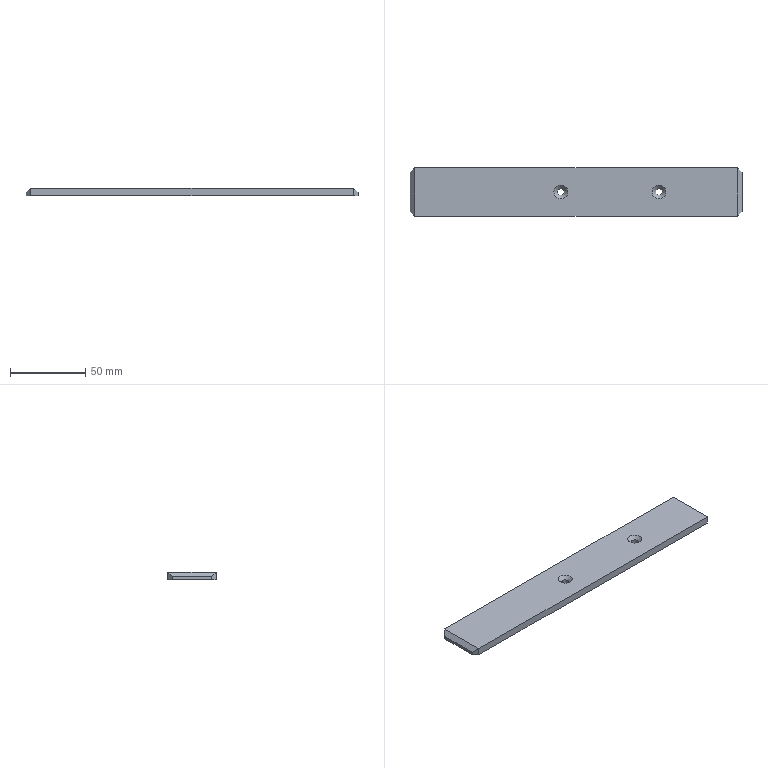Part | STEP file | Tube feed_id354_x_t | 1 solid | 16 faces | box 220 x 32 x 5 mm | volume 34590 mm3 | plane 12 | cone 2 | cylinder 2 | commonest cylinder face diameters 4.6 x2
STEP:
#1=CARTESIAN_POINT('',(0.,0.,0.));
#2=DIRECTION('',(0.,0.,1.));
#3=DIRECTION('',(1.,0.,0.));
#4=AXIS2_PLACEMENT_3D('',#1,#2,#3);
#5=CARTESIAN_POINT('',(203.,398.936,-4.));
#6=VERTEX_POINT('',#5);
#7=CARTESIAN_POINT('',(203.,424.936,-4.));
#8=VERTEX_POINT('',#7);
#9=CARTESIAN_POINT('',(203.,427.936,-4.));
#10=DIRECTION('',(0.,1.,0.));
#11=VECTOR('',#10,1.);
#12=LINE('',#9,#11);
#13=CARTESIAN_POINT('',(203.,427.936,-1.));
#14=DIRECTION('',(1.,0.,0.));
#15=DIRECTION('',(0.,0.,-1.));
#16=AXIS2_PLACEMENT_3D('',#13,#14,#15);
#17=PLANE('',#16);
#18=CARTESIAN_POINT('',(3.,0.));
#19=DIRECTION('',(0.,1.));
#20=VECTOR('',#19,1.);
#21=LINE('',#18,#20);
#22=(GEOMETRIC_REPRESENTATION_CONTEXT(2)PARAMETRIC_REPRESENTATION_CONTEXT()REPRESENTATION_CONTEXT('',''));
#23=DEFINITIONAL_REPRESENTATION('',(#21),#22);
#24=PCURVE('',#17,#23);
#25=CARTESIAN_POINT('',(206.,0.,-1.));
#26=DIRECTION('',(-0.7071,0.,0.7071));
#27=DIRECTION('',(0.,1.,0.));
#28=AXIS2_PLACEMENT_3D('',#25,#26,#27);
#29=PLANE('',#28);
#30=CARTESIAN_POINT('',(427.936,4.243));
#31=DIRECTION('',(1.,0.));
#32=VECTOR('',#31,1.);
#33=LINE('',#30,#32);
#34=(GEOMETRIC_REPRESENTATION_CONTEXT(2)PARAMETRIC_REPRESENTATION_CONTEXT()REPRESENTATION_CONTEXT('',''));
#35=DEFINITIONAL_REPRESENTATION('',(#33),#34);
#36=PCURVE('',#29,#35);
#37=SURFACE_CURVE('',#12,(#24,#36),.PCURVE_S1.);
#38=EDGE_CURVE('',#6,#8,#37,.T.);
#39=ORIENTED_EDGE('',*,*,#38,.T.);
#40=CARTESIAN_POINT('',(203.,424.936,-6.));
#41=VERTEX_POINT('',#40);
#42=CARTESIAN_POINT('',(203.,424.936,-1.));
#43=DIRECTION('',(0.,0.,-1.));
#44=VECTOR('',#43,1.);
#45=LINE('',#42,#44);
#46=CARTESIAN_POINT('',(0.,-3.));
#47=DIRECTION('',(1.,0.));
#48=VECTOR('',#47,1.);
#49=LINE('',#46,#48);
#50=(GEOMETRIC_REPRESENTATION_CONTEXT(2)PARAMETRIC_REPRESENTATION_CONTEXT()REPRESENTATION_CONTEXT('',''));
#51=DEFINITIONAL_REPRESENTATION('',(#49),#50);
#52=PCURVE('',#17,#51);
#53=CARTESIAN_POINT('',(203.,424.936,-1.));
#54=DIRECTION('',(0.7071,-0.7071,0.));
#55=DIRECTION('',(0.,0.,-1.));
#56=AXIS2_PLACEMENT_3D('',#53,#54,#55);
#57=PLANE('',#56);
#58=CARTESIAN_POINT('',(0.,0.));
#59=DIRECTION('',(1.,0.));
#60=VECTOR('',#59,1.);
#61=LINE('',#58,#60);
#62=(GEOMETRIC_REPRESENTATION_CONTEXT(2)PARAMETRIC_REPRESENTATION_CONTEXT()REPRESENTATION_CONTEXT('',''));
#63=DEFINITIONAL_REPRESENTATION('',(#61),#62);
#64=PCURVE('',#57,#63);
#65=SURFACE_CURVE('',#45,(#52,#64),.PCURVE_S1.);
#66=EDGE_CURVE('',#8,#41,#65,.T.);
#67=ORIENTED_EDGE('',*,*,#66,.T.);
#68=CARTESIAN_POINT('',(203.,398.936,-6.));
#69=VERTEX_POINT('',#68);
#70=CARTESIAN_POINT('',(203.,427.936,-6.));
#71=DIRECTION('',(0.,-1.,0.));
#72=VECTOR('',#71,1.);
#73=LINE('',#70,#72);
#74=CARTESIAN_POINT('',(5.,0.));
#75=DIRECTION('',(0.,-1.));
#76=VECTOR('',#75,1.);
#77=LINE('',#74,#76);
#78=(GEOMETRIC_REPRESENTATION_CONTEXT(2)PARAMETRIC_REPRESENTATION_CONTEXT()REPRESENTATION_CONTEXT('',''));
#79=DEFINITIONAL_REPRESENTATION('',(#77),#78);
#80=PCURVE('',#17,#79);
#81=CARTESIAN_POINT('',(0.,0.,-6.));
#82=DIRECTION('',(0.,0.,1.));
#83=DIRECTION('',(0.,-1.,0.));
#84=AXIS2_PLACEMENT_3D('',#81,#82,#83);
#85=PLANE('',#84);
#86=CARTESIAN_POINT('',(-427.936,203.));
#87=DIRECTION('',(1.,0.));
#88=VECTOR('',#87,1.);
#89=LINE('',#86,#88);
#90=(GEOMETRIC_REPRESENTATION_CONTEXT(2)PARAMETRIC_REPRESENTATION_CONTEXT()REPRESENTATION_CONTEXT('',''));
#91=DEFINITIONAL_REPRESENTATION('',(#89),#90);
#92=PCURVE('',#85,#91);
#93=SURFACE_CURVE('',#73,(#80,#92),.PCURVE_S1.);
#94=EDGE_CURVE('',#41,#69,#93,.T.);
#95=ORIENTED_EDGE('',*,*,#94,.T.);
#96=CARTESIAN_POINT('',(203.,398.936,-1.));
#97=DIRECTION('',(0.,0.,1.));
#98=VECTOR('',#97,1.);
#99=LINE('',#96,#98);
#100=CARTESIAN_POINT('',(0.,-29.));
#101=DIRECTION('',(-1.,0.));
#102=VECTOR('',#101,1.);
#103=LINE('',#100,#102);
#104=(GEOMETRIC_REPRESENTATION_CONTEXT(2)PARAMETRIC_REPRESENTATION_CONTEXT()REPRESENTATION_CONTEXT('',''));
#105=DEFINITIONAL_REPRESENTATION('',(#103),#104);
#106=PCURVE('',#17,#105);
#107=CARTESIAN_POINT('',(206.,395.936,-1.));
#108=DIRECTION('',(0.7071,0.7071,0.));
#109=DIRECTION('',(0.,0.,-1.));
#110=AXIS2_PLACEMENT_3D('',#107,#108,#109);
#111=PLANE('',#110);
#112=CARTESIAN_POINT('',(0.,4.243));
#113=DIRECTION('',(-1.,0.));
#114=VECTOR('',#113,1.);
#115=LINE('',#112,#114);
#116=(GEOMETRIC_REPRESENTATION_CONTEXT(2)PARAMETRIC_REPRESENTATION_CONTEXT()REPRESENTATION_CONTEXT('',''));
#117=DEFINITIONAL_REPRESENTATION('',(#115),#116);
#118=PCURVE('',#111,#117);
#119=SURFACE_CURVE('',#99,(#106,#118),.PCURVE_S1.);
#120=EDGE_CURVE('',#69,#6,#119,.T.);
#121=ORIENTED_EDGE('',*,*,#120,.T.);
#122=EDGE_LOOP('',(#39,#67,#95,#121));
#123=FACE_BOUND('',#122,.T.);
#124=ADVANCED_FACE('',(#123),#17,.F.);
#125=CARTESIAN_POINT('',(206.,395.936,-1.));
#126=VERTEX_POINT('',#125);
#127=CARTESIAN_POINT('',(420.,395.936,-1.));
#128=VERTEX_POINT('',#127);
#129=CARTESIAN_POINT('',(203.,395.936,-1.));
#130=DIRECTION('',(1.,0.,0.));
#131=VECTOR('',#130,1.);
#132=LINE('',#129,#131);
#133=CARTESIAN_POINT('',(203.,395.936,-1.));
#134=DIRECTION('',(0.,1.,0.));
#135=DIRECTION('',(0.,0.,1.));
#136=AXIS2_PLACEMENT_3D('',#133,#134,#135);
#137=PLANE('',#136);
#138=CARTESIAN_POINT('',(0.,0.));
#139=DIRECTION('',(0.,1.));
#140=VECTOR('',#139,1.);
#141=LINE('',#138,#140);
#142=(GEOMETRIC_REPRESENTATION_CONTEXT(2)PARAMETRIC_REPRESENTATION_CONTEXT()REPRESENTATION_CONTEXT('',''));
#143=DEFINITIONAL_REPRESENTATION('',(#141),#142);
#144=PCURVE('',#137,#143);
#145=CARTESIAN_POINT('',(0.,0.,-1.));
#146=DIRECTION('',(0.,0.,1.));
#147=DIRECTION('',(0.,-1.,0.));
#148=AXIS2_PLACEMENT_3D('',#145,#146,#147);
#149=PLANE('',#148);
#150=CARTESIAN_POINT('',(-395.936,203.));
#151=DIRECTION('',(0.,1.));
#152=VECTOR('',#151,1.);
#153=LINE('',#150,#152);
#154=(GEOMETRIC_REPRESENTATION_CONTEXT(2)PARAMETRIC_REPRESENTATION_CONTEXT()REPRESENTATION_CONTEXT('',''));
#155=DEFINITIONAL_REPRESENTATION('',(#153),#154);
#156=PCURVE('',#149,#155);
#157=SURFACE_CURVE('',#132,(#144,#156),.PCURVE_S1.);
#158=EDGE_CURVE('',#126,#128,#157,.T.);
#159=ORIENTED_EDGE('',*,*,#158,.F.);
#160=CARTESIAN_POINT('',(206.,395.936,-6.));
#161=VERTEX_POINT('',#160);
#162=CARTESIAN_POINT('',(206.,395.936,-1.));
#163=DIRECTION('',(0.,0.,-1.));
#164=VECTOR('',#163,1.);
#165=LINE('',#162,#164);
#166=CARTESIAN_POINT('',(0.,3.));
#167=DIRECTION('',(-1.,0.));
#168=VECTOR('',#167,1.);
#169=LINE('',#166,#168);
#170=(GEOMETRIC_REPRESENTATION_CONTEXT(2)PARAMETRIC_REPRESENTATION_CONTEXT()REPRESENTATION_CONTEXT('',''));
#171=DEFINITIONAL_REPRESENTATION('',(#169),#170);
#172=PCURVE('',#137,#171);
#173=CARTESIAN_POINT('',(0.,0.));
#174=DIRECTION('',(1.,0.));
#175=VECTOR('',#174,1.);
#176=LINE('',#173,#175);
#177=(GEOMETRIC_REPRESENTATION_CONTEXT(2)PARAMETRIC_REPRESENTATION_CONTEXT()REPRESENTATION_CONTEXT('',''));
#178=DEFINITIONAL_REPRESENTATION('',(#176),#177);
#179=PCURVE('',#111,#178);
#180=SURFACE_CURVE('',#165,(#172,#179),.PCURVE_S1.);
#181=EDGE_CURVE('',#126,#161,#180,.T.);
#182=ORIENTED_EDGE('',*,*,#181,.T.);
#183=CARTESIAN_POINT('',(420.,395.936,-6.));
#184=VERTEX_POINT('',#183);
#185=CARTESIAN_POINT('',(203.,395.936,-6.));
#186=DIRECTION('',(1.,0.,0.));
#187=VECTOR('',#186,1.);
#188=LINE('',#185,#187);
#189=CARTESIAN_POINT('',(-5.,0.));
#190=DIRECTION('',(0.,1.));
#191=VECTOR('',#190,1.);
#192=LINE('',#189,#191);
#193=(GEOMETRIC_REPRESENTATION_CONTEXT(2)PARAMETRIC_REPRESENTATION_CONTEXT()REPRESENTATION_CONTEXT('',''));
#194=DEFINITIONAL_REPRESENTATION('',(#192),#193);
#195=PCURVE('',#137,#194);
#196=CARTESIAN_POINT('',(-395.936,203.));
#197=DIRECTION('',(0.,1.));
#198=VECTOR('',#197,1.);
#199=LINE('',#196,#198);
#200=(GEOMETRIC_REPRESENTATION_CONTEXT(2)PARAMETRIC_REPRESENTATION_CONTEXT()REPRESENTATION_CONTEXT('',''));
#201=DEFINITIONAL_REPRESENTATION('',(#199),#200);
#202=PCURVE('',#85,#201);
#203=SURFACE_CURVE('',#188,(#195,#202),.PCURVE_S1.);
#204=EDGE_CURVE('',#161,#184,#203,.T.);
#205=ORIENTED_EDGE('',*,*,#204,.T.);
#206=CARTESIAN_POINT('',(420.,395.936,-1.));
#207=DIRECTION('',(0.,0.,1.));
#208=VECTOR('',#207,1.);
#209=LINE('',#206,#208);
#210=CARTESIAN_POINT('',(0.,217.));
#211=DIRECTION('',(1.,0.));
#212=VECTOR('',#211,1.);
#213=LINE('',#210,#212);
#214=(GEOMETRIC_REPRESENTATION_CONTEXT(2)PARAMETRIC_REPRESENTATION_CONTEXT()REPRESENTATION_CONTEXT('',''));
#215=DEFINITIONAL_REPRESENTATION('',(#213),#214);
#216=PCURVE('',#137,#215);
#217=CARTESIAN_POINT('',(423.,398.936,-1.));
#218=DIRECTION('',(-0.7071,0.7071,0.));
#219=DIRECTION('',(0.,0.,-1.));
#220=AXIS2_PLACEMENT_3D('',#217,#218,#219);
#221=PLANE('',#220);
#222=CARTESIAN_POINT('',(0.,4.243));
#223=DIRECTION('',(-1.,0.));
#224=VECTOR('',#223,1.);
#225=LINE('',#222,#224);
#226=(GEOMETRIC_REPRESENTATION_CONTEXT(2)PARAMETRIC_REPRESENTATION_CONTEXT()REPRESENTATION_CONTEXT('',''));
#227=DEFINITIONAL_REPRESENTATION('',(#225),#226);
#228=PCURVE('',#221,#227);
#229=SURFACE_CURVE('',#209,(#216,#228),.PCURVE_S1.);
#230=EDGE_CURVE('',#184,#128,#229,.T.);
#231=ORIENTED_EDGE('',*,*,#230,.T.);
#232=EDGE_LOOP('',(#159,#182,#205,#231));
#233=FACE_BOUND('',#232,.T.);
#234=ADVANCED_FACE('',(#233),#137,.F.);
#235=CARTESIAN_POINT('',(423.,398.936,-6.));
#236=VERTEX_POINT('',#235);
#237=CARTESIAN_POINT('',(423.,424.936,-6.));
#238=VERTEX_POINT('',#237);
#239=CARTESIAN_POINT('',(423.,395.936,-6.));
#240=DIRECTION('',(0.,1.,0.));
#241=VECTOR('',#240,1.);
#242=LINE('',#239,#241);
#243=CARTESIAN_POINT('',(423.,395.936,-1.));
#244=DIRECTION('',(-1.,0.,0.));
#245=DIRECTION('',(0.,0.,1.));
#246=AXIS2_PLACEMENT_3D('',#243,#244,#245);
#247=PLANE('',#246);
#248=CARTESIAN_POINT('',(-5.,0.));
#249=DIRECTION('',(0.,1.));
#250=VECTOR('',#249,1.);
#251=LINE('',#248,#250);
#252=(GEOMETRIC_REPRESENTATION_CONTEXT(2)PARAMETRIC_REPRESENTATION_CONTEXT()REPRESENTATION_CONTEXT('',''));
#253=DEFINITIONAL_REPRESENTATION('',(#251),#252);
#254=PCURVE('',#247,#253);
#255=CARTESIAN_POINT('',(-395.936,423.));
#256=DIRECTION('',(-1.,0.));
#257=VECTOR('',#256,1.);
#258=LINE('',#255,#257);
#259=(GEOMETRIC_REPRESENTATION_CONTEXT(2)PARAMETRIC_REPRESENTATION_CONTEXT()REPRESENTATION_CONTEXT('',''));
#260=DEFINITIONAL_REPRESENTATION('',(#258),#259);
#261=PCURVE('',#85,#260);
#262=SURFACE_CURVE('',#242,(#254,#261),.PCURVE_S1.);
#263=EDGE_CURVE('',#236,#238,#262,.T.);
#264=ORIENTED_EDGE('',*,*,#263,.T.);
#265=CARTESIAN_POINT('',(423.,424.936,-4.));
#266=VERTEX_POINT('',#265);
#267=CARTESIAN_POINT('',(423.,424.936,-1.));
#268=DIRECTION('',(0.,0.,1.));
#269=VECTOR('',#268,1.);
#270=LINE('',#267,#269);
#271=CARTESIAN_POINT('',(0.,29.));
#272=DIRECTION('',(1.,0.));
#273=VECTOR('',#272,1.);
#274=LINE('',#271,#273);
#275=(GEOMETRIC_REPRESENTATION_CONTEXT(2)PARAMETRIC_REPRESENTATION_CONTEXT()REPRESENTATION_CONTEXT('',''));
#276=DEFINITIONAL_REPRESENTATION('',(#274),#275);
#277=PCURVE('',#247,#276);
#278=CARTESIAN_POINT('',(420.,427.936,-1.));
#279=DIRECTION('',(-0.7071,-0.7071,0.));
#280=DIRECTION('',(0.,0.,-1.));
#281=AXIS2_PLACEMENT_3D('',#278,#279,#280);
#282=PLANE('',#281);
#283=CARTESIAN_POINT('',(0.,4.243));
#284=DIRECTION('',(-1.,0.));
#285=VECTOR('',#284,1.);
#286=LINE('',#283,#285);
#287=(GEOMETRIC_REPRESENTATION_CONTEXT(2)PARAMETRIC_REPRESENTATION_CONTEXT()REPRESENTATION_CONTEXT('',''));
#288=DEFINITIONAL_REPRESENTATION('',(#286),#287);
#289=PCURVE('',#282,#288);
#290=SURFACE_CURVE('',#270,(#277,#289),.PCURVE_S1.);
#291=EDGE_CURVE('',#238,#266,#290,.T.);
#292=ORIENTED_EDGE('',*,*,#291,.T.);
#293=CARTESIAN_POINT('',(423.,398.936,-4.));
#294=VERTEX_POINT('',#293);
#295=CARTESIAN_POINT('',(423.,395.936,-4.));
#296=DIRECTION('',(0.,-1.,0.));
#297=VECTOR('',#296,1.);
#298=LINE('',#295,#297);
#299=CARTESIAN_POINT('',(-3.,0.));
#300=DIRECTION('',(0.,-1.));
#301=VECTOR('',#300,1.);
#302=LINE('',#299,#301);
#303=(GEOMETRIC_REPRESENTATION_CONTEXT(2)PARAMETRIC_REPRESENTATION_CONTEXT()REPRESENTATION_CONTEXT('',''));
#304=DEFINITIONAL_REPRESENTATION('',(#302),#303);
#305=PCURVE('',#247,#304);
#306=CARTESIAN_POINT('',(420.,0.,-1.));
#307=DIRECTION('',(0.7071,0.,0.7071));
#308=DIRECTION('',(0.,-1.,0.));
#309=AXIS2_PLACEMENT_3D('',#306,#307,#308);
#310=PLANE('',#309);
#311=CARTESIAN_POINT('',(-395.936,4.243));
#312=DIRECTION('',(1.,0.));
#313=VECTOR('',#312,1.);
#314=LINE('',#311,#313);
#315=(GEOMETRIC_REPRESENTATION_CONTEXT(2)PARAMETRIC_REPRESENTATION_CONTEXT()REPRESENTATION_CONTEXT('',''));
#316=DEFINITIONAL_REPRESENTATION('',(#314),#315);
#317=PCURVE('',#310,#316);
#318=SURFACE_CURVE('',#298,(#305,#317),.PCURVE_S1.);
#319=EDGE_CURVE('',#266,#294,#318,.T.);
#320=ORIENTED_EDGE('',*,*,#319,.T.);
#321=CARTESIAN_POINT('',(423.,398.936,-1.));
#322=DIRECTION('',(0.,0.,-1.));
#323=VECTOR('',#322,1.);
#324=LINE('',#321,#323);
#325=CARTESIAN_POINT('',(0.,3.));
#326=DIRECTION('',(-1.,0.));
#327=VECTOR('',#326,1.);
#328=LINE('',#325,#327);
#329=(GEOMETRIC_REPRESENTATION_CONTEXT(2)PARAMETRIC_REPRESENTATION_CONTEXT()REPRESENTATION_CONTEXT('',''));
#330=DEFINITIONAL_REPRESENTATION('',(#328),#329);
#331=PCURVE('',#247,#330);
#332=CARTESIAN_POINT('',(0.,0.));
#333=DIRECTION('',(1.,0.));
#334=VECTOR('',#333,1.);
#335=LINE('',#332,#334);
#336=(GEOMETRIC_REPRESENTATION_CONTEXT(2)PARAMETRIC_REPRESENTATION_CONTEXT()REPRESENTATION_CONTEXT('',''));
#337=DEFINITIONAL_REPRESENTATION('',(#335),#336);
#338=PCURVE('',#221,#337);
#339=SURFACE_CURVE('',#324,(#331,#338),.PCURVE_S1.);
#340=EDGE_CURVE('',#294,#236,#339,.T.);
#341=ORIENTED_EDGE('',*,*,#340,.T.);
#342=EDGE_LOOP('',(#264,#292,#320,#341));
#343=FACE_BOUND('',#342,.T.);
#344=ADVANCED_FACE('',(#343),#247,.F.);
#345=CARTESIAN_POINT('',(420.,427.936,-6.));
#346=VERTEX_POINT('',#345);
#347=CARTESIAN_POINT('',(206.,427.936,-6.));
#348=VERTEX_POINT('',#347);
#349=CARTESIAN_POINT('',(423.,427.936,-6.));
#350=DIRECTION('',(-1.,0.,0.));
#351=VECTOR('',#350,1.);
#352=LINE('',#349,#351);
#353=CARTESIAN_POINT('',(423.,427.936,-1.));
#354=DIRECTION('',(0.,-1.,0.));
#355=DIRECTION('',(0.,0.,-1.));
#356=AXIS2_PLACEMENT_3D('',#353,#354,#355);
#357=PLANE('',#356);
#358=CARTESIAN_POINT('',(5.,0.));
#359=DIRECTION('',(0.,-1.));
#360=VECTOR('',#359,1.);
#361=LINE('',#358,#360);
#362=(GEOMETRIC_REPRESENTATION_CONTEXT(2)PARAMETRIC_REPRESENTATION_CONTEXT()REPRESENTATION_CONTEXT('',''));
#363=DEFINITIONAL_REPRESENTATION('',(#361),#362);
#364=PCURVE('',#357,#363);
#365=CARTESIAN_POINT('',(-427.936,423.));
#366=DIRECTION('',(0.,-1.));
#367=VECTOR('',#366,1.);
#368=LINE('',#365,#367);
#369=(GEOMETRIC_REPRESENTATION_CONTEXT(2)PARAMETRIC_REPRESENTATION_CONTEXT()REPRESENTATION_CONTEXT('',''));
#370=DEFINITIONAL_REPRESENTATION('',(#368),#369);
#371=PCURVE('',#85,#370);
#372=SURFACE_CURVE('',#352,(#364,#371),.PCURVE_S1.);
#373=EDGE_CURVE('',#346,#348,#372,.T.);
#374=ORIENTED_EDGE('',*,*,#373,.T.);
#375=CARTESIAN_POINT('',(206.,427.936,-1.));
#376=VERTEX_POINT('',#375);
#377=CARTESIAN_POINT('',(206.,427.936,-1.));
#378=DIRECTION('',(0.,0.,1.));
#379=VECTOR('',#378,1.);
#380=LINE('',#377,#379);
#381=CARTESIAN_POINT('',(0.,-217.));
#382=DIRECTION('',(-1.,0.));
#383=VECTOR('',#382,1.);
#384=LINE('',#381,#383);
#385=(GEOMETRIC_REPRESENTATION_CONTEXT(2)PARAMETRIC_REPRESENTATION_CONTEXT()REPRESENTATION_CONTEXT('',''));
#386=DEFINITIONAL_REPRESENTATION('',(#384),#385);
#387=PCURVE('',#357,#386);
#388=CARTESIAN_POINT('',(0.,4.243));
#389=DIRECTION('',(-1.,0.));
#390=VECTOR('',#389,1.);
#391=LINE('',#388,#390);
#392=(GEOMETRIC_REPRESENTATION_CONTEXT(2)PARAMETRIC_REPRESENTATION_CONTEXT()REPRESENTATION_CONTEXT('',''));
#393=DEFINITIONAL_REPRESENTATION('',(#391),#392);
#394=PCURVE('',#57,#393);
#395=SURFACE_CURVE('',#380,(#387,#394),.PCURVE_S1.);
#396=EDGE_CURVE('',#348,#376,#395,.T.);
#397=ORIENTED_EDGE('',*,*,#396,.T.);
#398=CARTESIAN_POINT('',(420.,427.936,-1.));
#399=VERTEX_POINT('',#398);
#400=CARTESIAN_POINT('',(423.,427.936,-1.));
#401=DIRECTION('',(-1.,0.,0.));
#402=VECTOR('',#401,1.);
#403=LINE('',#400,#402);
#404=CARTESIAN_POINT('',(0.,0.));
#405=DIRECTION('',(0.,-1.));
#406=VECTOR('',#405,1.);
#407=LINE('',#404,#406);
#408=(GEOMETRIC_REPRESENTATION_CONTEXT(2)PARAMETRIC_REPRESENTATION_CONTEXT()REPRESENTATION_CONTEXT('',''));
#409=DEFINITIONAL_REPRESENTATION('',(#407),#408);
#410=PCURVE('',#357,#409);
#411=CARTESIAN_POINT('',(-427.936,423.));
#412=DIRECTION('',(0.,-1.));
#413=VECTOR('',#412,1.);
#414=LINE('',#411,#413);
#415=(GEOMETRIC_REPRESENTATION_CONTEXT(2)PARAMETRIC_REPRESENTATION_CONTEXT()REPRESENTATION_CONTEXT('',''));
#416=DEFINITIONAL_REPRESENTATION('',(#414),#415);
#417=PCURVE('',#149,#416);
#418=SURFACE_CURVE('',#403,(#410,#417),.PCURVE_S1.);
#419=EDGE_CURVE('',#399,#376,#418,.T.);
#420=ORIENTED_EDGE('',*,*,#419,.F.);
#421=CARTESIAN_POINT('',(420.,427.936,-1.));
#422=DIRECTION('',(0.,0.,-1.));
#423=VECTOR('',#422,1.);
#424=LINE('',#421,#423);
#425=CARTESIAN_POINT('',(0.,-3.));
#426=DIRECTION('',(1.,0.));
#427=VECTOR('',#426,1.);
#428=LINE('',#425,#427);
#429=(GEOMETRIC_REPRESENTATION_CONTEXT(2)PARAMETRIC_REPRESENTATION_CONTEXT()REPRESENTATION_CONTEXT('',''));
#430=DEFINITIONAL_REPRESENTATION('',(#428),#429);
#431=PCURVE('',#357,#430);
#432=CARTESIAN_POINT('',(0.,0.));
#433=DIRECTION('',(1.,0.));
#434=VECTOR('',#433,1.);
#435=LINE('',#432,#434);
#436=(GEOMETRIC_REPRESENTATION_CONTEXT(2)PARAMETRIC_REPRESENTATION_CONTEXT()REPRESENTATION_CONTEXT('',''));
#437=DEFINITIONAL_REPRESENTATION('',(#435),#436);
#438=PCURVE('',#282,#437);
#439=SURFACE_CURVE('',#424,(#431,#438),.PCURVE_S1.);
#440=EDGE_CURVE('',#399,#346,#439,.T.);
#441=ORIENTED_EDGE('',*,*,#440,.T.);
#442=EDGE_LOOP('',(#374,#397,#420,#441));
#443=FACE_BOUND('',#442,.T.);
#444=ADVANCED_FACE('',(#443),#357,.F.);
#445=CARTESIAN_POINT('',(363.4,411.936,-1.));
#446=VERTEX_POINT('',#445);
#447=CARTESIAN_POINT('',(368.,411.936,-1.));
#448=DIRECTION('',(0.,0.,-1.));
#449=DIRECTION('',(-1.,0.,0.));
#450=AXIS2_PLACEMENT_3D('',#447,#448,#449);
#451=CIRCLE('',#450,4.6);
#452=CARTESIAN_POINT('',(-411.936,363.4));
#453=CARTESIAN_POINT('',(-419.903,363.4));
#454=CARTESIAN_POINT('',(-415.919,370.3));
#455=CARTESIAN_POINT('',(-411.936,377.2));
#456=CARTESIAN_POINT('',(-407.952,370.3));
#457=CARTESIAN_POINT('',(-403.968,363.4));
#458=CARTESIAN_POINT('',(-411.936,363.4));
#459=(BOUNDED_CURVE()B_SPLINE_CURVE(2,(#452,#453,#454,#455,#456,#457,#458),.UNSPECIFIED.,.T.,.F.)B_SPLINE_CURVE_WITH_KNOTS((1,2,2,2,2,1),(-2.094,0.,2.094,4.189,6.283,8.378),.UNSPECIFIED.)CURVE()GEOMETRIC_REPRESENTATION_ITEM()RATIONAL_B_SPLINE_CURVE((1.,0.5,1.,0.5,1.,0.5,1.))REPRESENTATION_ITEM(''));
#460=(GEOMETRIC_REPRESENTATION_CONTEXT(2)PARAMETRIC_REPRESENTATION_CONTEXT()REPRESENTATION_CONTEXT('',''));
#461=DEFINITIONAL_REPRESENTATION('',(#459),#460);
#462=PCURVE('',#149,#461);
#463=CARTESIAN_POINT('',(368.,411.936,-3.3));
#464=DIRECTION('',(0.,0.,1.));
#465=DIRECTION('',(1.,0.,0.));
#466=AXIS2_PLACEMENT_3D('',#463,#464,#465);
#467=CONICAL_SURFACE('',#466,2.3,0.7854);
#468=CARTESIAN_POINT('',(9.425,2.3));
#469=DIRECTION('',(-1.,0.));
#470=VECTOR('',#469,1.);
#471=LINE('',#468,#470);
#472=(GEOMETRIC_REPRESENTATION_CONTEXT(2)PARAMETRIC_REPRESENTATION_CONTEXT()REPRESENTATION_CONTEXT('',''));
#473=DEFINITIONAL_REPRESENTATION('',(#471),#472);
#474=PCURVE('',#467,#473);
#475=SURFACE_CURVE('',#451,(#462,#474),.PCURVE_S1.);
#476=EDGE_CURVE('',#446,#446,#475,.T.);
#477=ORIENTED_EDGE('',*,*,#476,.T.);
#478=EDGE_LOOP('',(#477));
#479=FACE_BOUND('',#478,.T.);
#480=CARTESIAN_POINT('',(298.4,411.936,-1.));
#481=VERTEX_POINT('',#480);
#482=CARTESIAN_POINT('',(303.,411.936,-1.));
#483=DIRECTION('',(0.,0.,-1.));
#484=DIRECTION('',(-1.,0.,0.));
#485=AXIS2_PLACEMENT_3D('',#482,#483,#484);
#486=CIRCLE('',#485,4.6);
#487=CARTESIAN_POINT('',(-411.936,298.4));
#488=CARTESIAN_POINT('',(-419.903,298.4));
#489=CARTESIAN_POINT('',(-415.919,305.3));
#490=CARTESIAN_POINT('',(-411.936,312.2));
#491=CARTESIAN_POINT('',(-407.952,305.3));
#492=CARTESIAN_POINT('',(-403.968,298.4));
#493=CARTESIAN_POINT('',(-411.936,298.4));
#494=(BOUNDED_CURVE()B_SPLINE_CURVE(2,(#487,#488,#489,#490,#491,#492,#493),.UNSPECIFIED.,.T.,.F.)B_SPLINE_CURVE_WITH_KNOTS((1,2,2,2,2,1),(-2.094,0.,2.094,4.189,6.283,8.378),.UNSPECIFIED.)CURVE()GEOMETRIC_REPRESENTATION_ITEM()RATIONAL_B_SPLINE_CURVE((1.,0.5,1.,0.5,1.,0.5,1.))REPRESENTATION_ITEM(''));
#495=(GEOMETRIC_REPRESENTATION_CONTEXT(2)PARAMETRIC_REPRESENTATION_CONTEXT()REPRESENTATION_CONTEXT('',''));
#496=DEFINITIONAL_REPRESENTATION('',(#494),#495);
#497=PCURVE('',#149,#496);
#498=CARTESIAN_POINT('',(303.,411.936,-3.3));
#499=DIRECTION('',(0.,0.,1.));
#500=DIRECTION('',(1.,0.,0.));
#501=AXIS2_PLACEMENT_3D('',#498,#499,#500);
#502=CONICAL_SURFACE('',#501,2.3,0.7854);
#503=CARTESIAN_POINT('',(9.425,2.3));
#504=DIRECTION('',(-1.,0.));
#505=VECTOR('',#504,1.);
#506=LINE('',#503,#505);
#507=(GEOMETRIC_REPRESENTATION_CONTEXT(2)PARAMETRIC_REPRESENTATION_CONTEXT()REPRESENTATION_CONTEXT('',''));
#508=DEFINITIONAL_REPRESENTATION('',(#506),#507);
#509=PCURVE('',#502,#508);
#510=SURFACE_CURVE('',#486,(#497,#509),.PCURVE_S1.);
#511=EDGE_CURVE('',#481,#481,#510,.T.);
#512=ORIENTED_EDGE('',*,*,#511,.T.);
#513=EDGE_LOOP('',(#512));
#514=FACE_BOUND('',#513,.T.);
#515=ORIENTED_EDGE('',*,*,#419,.T.);
#516=CARTESIAN_POINT('',(206.,395.936,-1.));
#517=DIRECTION('',(0.,-1.,0.));
#518=VECTOR('',#517,1.);
#519=LINE('',#516,#518);
#520=CARTESIAN_POINT('',(-395.936,206.));
#521=DIRECTION('',(1.,0.));
#522=VECTOR('',#521,1.);
#523=LINE('',#520,#522);
#524=(GEOMETRIC_REPRESENTATION_CONTEXT(2)PARAMETRIC_REPRESENTATION_CONTEXT()REPRESENTATION_CONTEXT('',''));
#525=DEFINITIONAL_REPRESENTATION('',(#523),#524);
#526=PCURVE('',#149,#525);
#527=CARTESIAN_POINT('',(395.936,0.));
#528=DIRECTION('',(-1.,0.));
#529=VECTOR('',#528,1.);
#530=LINE('',#527,#529);
#531=(GEOMETRIC_REPRESENTATION_CONTEXT(2)PARAMETRIC_REPRESENTATION_CONTEXT()REPRESENTATION_CONTEXT('',''));
#532=DEFINITIONAL_REPRESENTATION('',(#530),#531);
#533=PCURVE('',#29,#532);
#534=SURFACE_CURVE('',#519,(#526,#533),.PCURVE_S1.);
#535=EDGE_CURVE('',#376,#126,#534,.T.);
#536=ORIENTED_EDGE('',*,*,#535,.T.);
#537=ORIENTED_EDGE('',*,*,#158,.T.);
#538=CARTESIAN_POINT('',(420.,427.936,-1.));
#539=DIRECTION('',(0.,1.,0.));
#540=VECTOR('',#539,1.);
#541=LINE('',#538,#540);
#542=CARTESIAN_POINT('',(-427.936,420.));
#543=DIRECTION('',(-1.,0.));
#544=VECTOR('',#543,1.);
#545=LINE('',#542,#544);
#546=(GEOMETRIC_REPRESENTATION_CONTEXT(2)PARAMETRIC_REPRESENTATION_CONTEXT()REPRESENTATION_CONTEXT('',''));
#547=DEFINITIONAL_REPRESENTATION('',(#545),#546);
#548=PCURVE('',#149,#547);
#549=CARTESIAN_POINT('',(-427.936,0.));
#550=DIRECTION('',(-1.,0.));
#551=VECTOR('',#550,1.);
#552=LINE('',#549,#551);
#553=(GEOMETRIC_REPRESENTATION_CONTEXT(2)PARAMETRIC_REPRESENTATION_CONTEXT()REPRESENTATION_CONTEXT('',''));
#554=DEFINITIONAL_REPRESENTATION('',(#552),#553);
#555=PCURVE('',#310,#554);
#556=SURFACE_CURVE('',#541,(#548,#555),.PCURVE_S1.);
#557=EDGE_CURVE('',#128,#399,#556,.T.);
#558=ORIENTED_EDGE('',*,*,#557,.T.);
#559=EDGE_LOOP('',(#515,#536,#537,#558));
#560=FACE_BOUND('',#559,.T.);
#561=ADVANCED_FACE('',(#479,#514,#560),#149,.T.);
#562=CARTESIAN_POINT('',(368.,409.636,-6.));
#563=VERTEX_POINT('',#562);
#564=CARTESIAN_POINT('',(365.7,411.936,-6.));
#565=VERTEX_POINT('',#564);
#566=CARTESIAN_POINT('',(368.,411.936,-6.));
#567=DIRECTION('',(0.,0.,-1.));
#568=DIRECTION('',(0.,-1.,0.));
#569=AXIS2_PLACEMENT_3D('',#566,#567,#568);
#570=CIRCLE('',#569,2.3);
#571=CARTESIAN_POINT('',(-409.636,368.));
#572=CARTESIAN_POINT('',(-409.636,364.016));
#573=CARTESIAN_POINT('',(-413.086,366.008));
#574=CARTESIAN_POINT('',(-416.536,368.));
#575=CARTESIAN_POINT('',(-413.086,369.992));
#576=CARTESIAN_POINT('',(-409.636,371.984));
#577=CARTESIAN_POINT('',(-409.636,368.));
#578=(BOUNDED_CURVE()B_SPLINE_CURVE(2,(#571,#572,#573,#574,#575,#576,#577),.UNSPECIFIED.,.T.,.F.)B_SPLINE_CURVE_WITH_KNOTS((1,2,2,2,2,1),(-2.094,0.,2.094,4.189,6.283,8.378),.UNSPECIFIED.)CURVE()GEOMETRIC_REPRESENTATION_ITEM()RATIONAL_B_SPLINE_CURVE((1.,0.5,1.,0.5,1.,0.5,1.))REPRESENTATION_ITEM(''));
#579=(GEOMETRIC_REPRESENTATION_CONTEXT(2)PARAMETRIC_REPRESENTATION_CONTEXT()REPRESENTATION_CONTEXT('',''));
#580=DEFINITIONAL_REPRESENTATION('',(#578),#579);
#581=PCURVE('',#85,#580);
#582=CARTESIAN_POINT('',(368.,411.936,-16.6));
#583=DIRECTION('',(0.,0.,-1.));
#584=DIRECTION('',(-1.,0.,0.));
#585=AXIS2_PLACEMENT_3D('',#582,#583,#584);
#586=CYLINDRICAL_SURFACE('',#585,2.3);
#587=CARTESIAN_POINT('',(4.712,-10.6));
#588=DIRECTION('',(1.,0.));
#589=VECTOR('',#588,1.);
#590=LINE('',#587,#589);
#591=(GEOMETRIC_REPRESENTATION_CONTEXT(2)PARAMETRIC_REPRESENTATION_CONTEXT()REPRESENTATION_CONTEXT('',''));
#592=DEFINITIONAL_REPRESENTATION('',(#590),#591);
#593=PCURVE('',#586,#592);
#594=SURFACE_CURVE('',#570,(#581,#593),.PCURVE_S1.);
#595=EDGE_CURVE('',#563,#565,#594,.T.);
#596=ORIENTED_EDGE('',*,*,#595,.F.);
#597=CARTESIAN_POINT('',(368.,411.936,-6.));
#598=DIRECTION('',(0.,0.,-1.));
#599=DIRECTION('',(0.,-1.,0.));
#600=AXIS2_PLACEMENT_3D('',#597,#598,#599);
#601=CIRCLE('',#600,2.3);
#602=CARTESIAN_POINT('',(-409.636,368.));
#603=CARTESIAN_POINT('',(-409.636,364.016));
#604=CARTESIAN_POINT('',(-413.086,366.008));
#605=CARTESIAN_POINT('',(-416.536,368.));
#606=CARTESIAN_POINT('',(-413.086,369.992));
#607=CARTESIAN_POINT('',(-409.636,371.984));
#608=CARTESIAN_POINT('',(-409.636,368.));
#609=(BOUNDED_CURVE()B_SPLINE_CURVE(2,(#602,#603,#604,#605,#606,#607,#608),.UNSPECIFIED.,.T.,.F.)B_SPLINE_CURVE_WITH_KNOTS((1,2,2,2,2,1),(-2.094,0.,2.094,4.189,6.283,8.378),.UNSPECIFIED.)CURVE()GEOMETRIC_REPRESENTATION_ITEM()RATIONAL_B_SPLINE_CURVE((1.,0.5,1.,0.5,1.,0.5,1.))REPRESENTATION_ITEM(''));
#610=(GEOMETRIC_REPRESENTATION_CONTEXT(2)PARAMETRIC_REPRESENTATION_CONTEXT()REPRESENTATION_CONTEXT('',''));
#611=DEFINITIONAL_REPRESENTATION('',(#609),#610);
#612=PCURVE('',#85,#611);
#613=CARTESIAN_POINT('',(-1.571,-10.6));
#614=DIRECTION('',(1.,0.));
#615=VECTOR('',#614,1.);
#616=LINE('',#613,#615);
#617=(GEOMETRIC_REPRESENTATION_CONTEXT(2)PARAMETRIC_REPRESENTATION_CONTEXT()REPRESENTATION_CONTEXT('',''));
#618=DEFINITIONAL_REPRESENTATION('',(#616),#617);
#619=PCURVE('',#586,#618);
#620=SURFACE_CURVE('',#601,(#612,#619),.PCURVE_S1.);
#621=EDGE_CURVE('',#565,#563,#620,.T.);
#622=ORIENTED_EDGE('',*,*,#621,.F.);
#623=EDGE_LOOP('',(#596,#622));
#624=FACE_BOUND('',#623,.T.);
#625=CARTESIAN_POINT('',(303.,409.636,-6.));
#626=VERTEX_POINT('',#625);
#627=CARTESIAN_POINT('',(300.7,411.936,-6.));
#628=VERTEX_POINT('',#627);
#629=CARTESIAN_POINT('',(303.,411.936,-6.));
#630=DIRECTION('',(0.,0.,1.));
#631=DIRECTION('',(0.,-1.,0.));
#632=AXIS2_PLACEMENT_3D('',#629,#630,#631);
#633=CIRCLE('',#632,2.3);
#634=CARTESIAN_POINT('',(-411.936,303.));
#635=DIRECTION('',(1.,0.));
#636=AXIS2_PLACEMENT_2D('',#634,#635);
#637=CIRCLE('',#636,2.3);
#638=(GEOMETRIC_REPRESENTATION_CONTEXT(2)PARAMETRIC_REPRESENTATION_CONTEXT()REPRESENTATION_CONTEXT('',''));
#639=DEFINITIONAL_REPRESENTATION('',(#637),#638);
#640=PCURVE('',#85,#639);
#641=CARTESIAN_POINT('',(303.,411.936,-17.3));
#642=DIRECTION('',(0.,0.,-1.));
#643=DIRECTION('',(-1.,0.,0.));
#644=AXIS2_PLACEMENT_3D('',#641,#642,#643);
#645=CYLINDRICAL_SURFACE('',#644,2.3);
#646=CARTESIAN_POINT('',(4.712,-11.3));
#647=DIRECTION('',(-1.,0.));
#648=VECTOR('',#647,1.);
#649=LINE('',#646,#648);
#650=(GEOMETRIC_REPRESENTATION_CONTEXT(2)PARAMETRIC_REPRESENTATION_CONTEXT()REPRESENTATION_CONTEXT('',''));
#651=DEFINITIONAL_REPRESENTATION('',(#649),#650);
#652=PCURVE('',#645,#651);
#653=SURFACE_CURVE('',#633,(#640,#652),.PCURVE_S1.);
#654=EDGE_CURVE('',#626,#628,#653,.T.);
#655=ORIENTED_EDGE('',*,*,#654,.T.);
#656=CARTESIAN_POINT('',(303.,411.936,-6.));
#657=DIRECTION('',(0.,0.,1.));
#658=DIRECTION('',(0.,-1.,0.));
#659=AXIS2_PLACEMENT_3D('',#656,#657,#658);
#660=CIRCLE('',#659,2.3);
#661=CARTESIAN_POINT('',(-411.936,303.));
#662=DIRECTION('',(1.,0.));
#663=AXIS2_PLACEMENT_2D('',#661,#662);
#664=CIRCLE('',#663,2.3);
#665=(GEOMETRIC_REPRESENTATION_CONTEXT(2)PARAMETRIC_REPRESENTATION_CONTEXT()REPRESENTATION_CONTEXT('',''));
#666=DEFINITIONAL_REPRESENTATION('',(#664),#665);
#667=PCURVE('',#85,#666);
#668=CARTESIAN_POINT('',(10.996,-11.3));
#669=DIRECTION('',(-1.,0.));
#670=VECTOR('',#669,1.);
#671=LINE('',#668,#670);
#672=(GEOMETRIC_REPRESENTATION_CONTEXT(2)PARAMETRIC_REPRESENTATION_CONTEXT()REPRESENTATION_CONTEXT('',''));
#673=DEFINITIONAL_REPRESENTATION('',(#671),#672);
#674=PCURVE('',#645,#673);
#675=SURFACE_CURVE('',#660,(#667,#674),.PCURVE_S1.);
#676=EDGE_CURVE('',#628,#626,#675,.T.);
#677=ORIENTED_EDGE('',*,*,#676,.T.);
#678=EDGE_LOOP('',(#655,#677));
#679=FACE_BOUND('',#678,.T.);
#680=ORIENTED_EDGE('',*,*,#94,.F.);
#681=CARTESIAN_POINT('',(203.,424.936,-6.));
#682=DIRECTION('',(0.7071,0.7071,0.));
#683=VECTOR('',#682,1.);
#684=LINE('',#681,#683);
#685=CARTESIAN_POINT('',(-424.936,203.));
#686=DIRECTION('',(-0.7071,0.7071));
#687=VECTOR('',#686,1.);
#688=LINE('',#685,#687);
#689=(GEOMETRIC_REPRESENTATION_CONTEXT(2)PARAMETRIC_REPRESENTATION_CONTEXT()REPRESENTATION_CONTEXT('',''));
#690=DEFINITIONAL_REPRESENTATION('',(#688),#689);
#691=PCURVE('',#85,#690);
#692=CARTESIAN_POINT('',(5.,0.));
#693=DIRECTION('',(0.,1.));
#694=VECTOR('',#693,1.);
#695=LINE('',#692,#694);
#696=(GEOMETRIC_REPRESENTATION_CONTEXT(2)PARAMETRIC_REPRESENTATION_CONTEXT()REPRESENTATION_CONTEXT('',''));
#697=DEFINITIONAL_REPRESENTATION('',(#695),#696);
#698=PCURVE('',#57,#697);
#699=SURFACE_CURVE('',#684,(#691,#698),.PCURVE_S1.);
#700=EDGE_CURVE('',#41,#348,#699,.T.);
#701=ORIENTED_EDGE('',*,*,#700,.T.);
#702=ORIENTED_EDGE('',*,*,#373,.F.);
#703=CARTESIAN_POINT('',(420.,427.936,-6.));
#704=DIRECTION('',(0.7071,-0.7071,0.));
#705=VECTOR('',#704,1.);
#706=LINE('',#703,#705);
#707=CARTESIAN_POINT('',(-427.936,420.));
#708=DIRECTION('',(0.7071,0.7071));
#709=VECTOR('',#708,1.);
#710=LINE('',#707,#709);
#711=(GEOMETRIC_REPRESENTATION_CONTEXT(2)PARAMETRIC_REPRESENTATION_CONTEXT()REPRESENTATION_CONTEXT('',''));
#712=DEFINITIONAL_REPRESENTATION('',(#710),#711);
#713=PCURVE('',#85,#712);
#714=CARTESIAN_POINT('',(5.,0.));
#715=DIRECTION('',(0.,1.));
#716=VECTOR('',#715,1.);
#717=LINE('',#714,#716);
#718=(GEOMETRIC_REPRESENTATION_CONTEXT(2)PARAMETRIC_REPRESENTATION_CONTEXT()REPRESENTATION_CONTEXT('',''));
#719=DEFINITIONAL_REPRESENTATION('',(#717),#718);
#720=PCURVE('',#282,#719);
#721=SURFACE_CURVE('',#706,(#713,#720),.PCURVE_S1.);
#722=EDGE_CURVE('',#346,#238,#721,.T.);
#723=ORIENTED_EDGE('',*,*,#722,.T.);
#724=ORIENTED_EDGE('',*,*,#263,.F.);
#725=CARTESIAN_POINT('',(423.,398.936,-6.));
#726=DIRECTION('',(-0.7071,-0.7071,0.));
#727=VECTOR('',#726,1.);
#728=LINE('',#725,#727);
#729=CARTESIAN_POINT('',(-398.936,423.));
#730=DIRECTION('',(0.7071,-0.7071));
#731=VECTOR('',#730,1.);
#732=LINE('',#729,#731);
#733=(GEOMETRIC_REPRESENTATION_CONTEXT(2)PARAMETRIC_REPRESENTATION_CONTEXT()REPRESENTATION_CONTEXT('',''));
#734=DEFINITIONAL_REPRESENTATION('',(#732),#733);
#735=PCURVE('',#85,#734);
#736=CARTESIAN_POINT('',(5.,0.));
#737=DIRECTION('',(0.,1.));
#738=VECTOR('',#737,1.);
#739=LINE('',#736,#738);
#740=(GEOMETRIC_REPRESENTATION_CONTEXT(2)PARAMETRIC_REPRESENTATION_CONTEXT()REPRESENTATION_CONTEXT('',''));
#741=DEFINITIONAL_REPRESENTATION('',(#739),#740);
#742=PCURVE('',#221,#741);
#743=SURFACE_CURVE('',#728,(#735,#742),.PCURVE_S1.);
#744=EDGE_CURVE('',#236,#184,#743,.T.);
#745=ORIENTED_EDGE('',*,*,#744,.T.);
#746=ORIENTED_EDGE('',*,*,#204,.F.);
#747=CARTESIAN_POINT('',(206.,395.936,-6.));
#748=DIRECTION('',(-0.7071,0.7071,0.));
#749=VECTOR('',#748,1.);
#750=LINE('',#747,#749);
#751=CARTESIAN_POINT('',(-395.936,206.));
#752=DIRECTION('',(-0.7071,-0.7071));
#753=VECTOR('',#752,1.);
#754=LINE('',#751,#753);
#755=(GEOMETRIC_REPRESENTATION_CONTEXT(2)PARAMETRIC_REPRESENTATION_CONTEXT()REPRESENTATION_CONTEXT('',''));
#756=DEFINITIONAL_REPRESENTATION('',(#754),#755);
#757=PCURVE('',#85,#756);
#758=CARTESIAN_POINT('',(5.,0.));
#759=DIRECTION('',(0.,1.));
#760=VECTOR('',#759,1.);
#761=LINE('',#758,#760);
#762=(GEOMETRIC_REPRESENTATION_CONTEXT(2)PARAMETRIC_REPRESENTATION_CONTEXT()REPRESENTATION_CONTEXT('',''));
#763=DEFINITIONAL_REPRESENTATION('',(#761),#762);
#764=PCURVE('',#111,#763);
#765=SURFACE_CURVE('',#750,(#757,#764),.PCURVE_S1.);
#766=EDGE_CURVE('',#161,#69,#765,.T.);
#767=ORIENTED_EDGE('',*,*,#766,.T.);
#768=EDGE_LOOP('',(#680,#701,#702,#723,#724,#745,#746,#767));
#769=FACE_BOUND('',#768,.T.);
#770=ADVANCED_FACE('',(#624,#679,#769),#85,.F.);
#771=ORIENTED_EDGE('',*,*,#766,.F.);
#772=ORIENTED_EDGE('',*,*,#181,.F.);
#773=CARTESIAN_POINT('',(206.,395.936,-1.));
#774=DIRECTION('',(0.5774,-0.5774,0.5774));
#775=VECTOR('',#774,1.);
#776=LINE('',#773,#775);
#777=CARTESIAN_POINT('',(0.,0.));
#778=DIRECTION('',(-0.5774,-0.8165));
#779=VECTOR('',#778,1.);
#780=LINE('',#777,#779);
#781=(GEOMETRIC_REPRESENTATION_CONTEXT(2)PARAMETRIC_REPRESENTATION_CONTEXT()REPRESENTATION_CONTEXT('',''));
#782=DEFINITIONAL_REPRESENTATION('',(#780),#781);
#783=PCURVE('',#111,#782);
#784=CARTESIAN_POINT('',(395.936,0.));
#785=DIRECTION('',(-0.5774,-0.8165));
#786=VECTOR('',#785,1.);
#787=LINE('',#784,#786);
#788=(GEOMETRIC_REPRESENTATION_CONTEXT(2)PARAMETRIC_REPRESENTATION_CONTEXT()REPRESENTATION_CONTEXT('',''));
#789=DEFINITIONAL_REPRESENTATION('',(#787),#788);
#790=PCURVE('',#29,#789);
#791=SURFACE_CURVE('',#776,(#783,#790),.PCURVE_S1.);
#792=EDGE_CURVE('',#6,#126,#791,.T.);
#793=ORIENTED_EDGE('',*,*,#792,.F.);
#794=ORIENTED_EDGE('',*,*,#120,.F.);
#795=EDGE_LOOP('',(#771,#772,#793,#794));
#796=FACE_BOUND('',#795,.T.);
#797=ADVANCED_FACE('',(#796),#111,.F.);
#798=ORIENTED_EDGE('',*,*,#792,.T.);
#799=ORIENTED_EDGE('',*,*,#535,.F.);
#800=CARTESIAN_POINT('',(63.355,285.29,-143.645));
#801=DIRECTION('',(0.5774,0.5774,0.5774));
#802=VECTOR('',#801,1.);
#803=LINE('',#800,#802);
#804=CARTESIAN_POINT('',(285.29,201.731));
#805=DIRECTION('',(0.5774,-0.8165));
#806=VECTOR('',#805,1.);
#807=LINE('',#804,#806);
#808=(GEOMETRIC_REPRESENTATION_CONTEXT(2)PARAMETRIC_REPRESENTATION_CONTEXT()REPRESENTATION_CONTEXT('',''));
#809=DEFINITIONAL_REPRESENTATION('',(#807),#808);
#810=PCURVE('',#29,#809);
#811=CARTESIAN_POINT('',(142.645,-197.488));
#812=DIRECTION('',(-0.5774,0.8165));
#813=VECTOR('',#812,1.);
#814=LINE('',#811,#813);
#815=(GEOMETRIC_REPRESENTATION_CONTEXT(2)PARAMETRIC_REPRESENTATION_CONTEXT()REPRESENTATION_CONTEXT('',''));
#816=DEFINITIONAL_REPRESENTATION('',(#814),#815);
#817=PCURVE('',#57,#816);
#818=SURFACE_CURVE('',#803,(#810,#817),.PCURVE_S1.);
#819=EDGE_CURVE('',#8,#376,#818,.T.);
#820=ORIENTED_EDGE('',*,*,#819,.F.);
#821=ORIENTED_EDGE('',*,*,#38,.F.);
#822=EDGE_LOOP('',(#798,#799,#820,#821));
#823=FACE_BOUND('',#822,.T.);
#824=ADVANCED_FACE('',(#823),#29,.T.);
#825=ORIENTED_EDGE('',*,*,#819,.T.);
#826=ORIENTED_EDGE('',*,*,#396,.F.);
#827=ORIENTED_EDGE('',*,*,#700,.F.);
#828=ORIENTED_EDGE('',*,*,#66,.F.);
#829=EDGE_LOOP('',(#825,#826,#827,#828));
#830=FACE_BOUND('',#829,.T.);
#831=ADVANCED_FACE('',(#830),#57,.F.);
#832=ORIENTED_EDGE('',*,*,#744,.F.);
#833=ORIENTED_EDGE('',*,*,#340,.F.);
#834=CARTESIAN_POINT('',(422.,397.936,-3.));
#835=DIRECTION('',(0.5774,0.5774,-0.5774));
#836=VECTOR('',#835,1.);
#837=LINE('',#834,#836);
#838=CARTESIAN_POINT('',(2.,1.414));
#839=DIRECTION('',(0.5774,-0.8165));
#840=VECTOR('',#839,1.);
#841=LINE('',#838,#840);
#842=(GEOMETRIC_REPRESENTATION_CONTEXT(2)PARAMETRIC_REPRESENTATION_CONTEXT()REPRESENTATION_CONTEXT('',''));
#843=DEFINITIONAL_REPRESENTATION('',(#841),#842);
#844=PCURVE('',#221,#843);
#845=CARTESIAN_POINT('',(-397.936,2.828));
#846=DIRECTION('',(-0.5774,0.8165));
#847=VECTOR('',#846,1.);
#848=LINE('',#845,#847);
#849=(GEOMETRIC_REPRESENTATION_CONTEXT(2)PARAMETRIC_REPRESENTATION_CONTEXT()REPRESENTATION_CONTEXT('',''));
#850=DEFINITIONAL_REPRESENTATION('',(#848),#849);
#851=PCURVE('',#310,#850);
#852=SURFACE_CURVE('',#837,(#844,#851),.PCURVE_S1.);
#853=EDGE_CURVE('',#128,#294,#852,.T.);
#854=ORIENTED_EDGE('',*,*,#853,.F.);
#855=ORIENTED_EDGE('',*,*,#230,.F.);
#856=EDGE_LOOP('',(#832,#833,#854,#855));
#857=FACE_BOUND('',#856,.T.);
#858=ADVANCED_FACE('',(#857),#221,.F.);
#859=ORIENTED_EDGE('',*,*,#853,.T.);
#860=ORIENTED_EDGE('',*,*,#319,.F.);
#861=CARTESIAN_POINT('',(562.645,285.29,-143.645));
#862=DIRECTION('',(0.5774,-0.5774,-0.5774));
#863=VECTOR('',#862,1.);
#864=LINE('',#861,#863);
#865=CARTESIAN_POINT('',(-285.29,201.731));
#866=DIRECTION('',(0.5774,0.8165));
#867=VECTOR('',#866,1.);
#868=LINE('',#865,#867);
#869=(GEOMETRIC_REPRESENTATION_CONTEXT(2)PARAMETRIC_REPRESENTATION_CONTEXT()REPRESENTATION_CONTEXT('',''));
#870=DEFINITIONAL_REPRESENTATION('',(#868),#869);
#871=PCURVE('',#310,#870);
#872=CARTESIAN_POINT('',(142.645,201.731));
#873=DIRECTION('',(0.5774,0.8165));
#874=VECTOR('',#873,1.);
#875=LINE('',#872,#874);
#876=(GEOMETRIC_REPRESENTATION_CONTEXT(2)PARAMETRIC_REPRESENTATION_CONTEXT()REPRESENTATION_CONTEXT('',''));
#877=DEFINITIONAL_REPRESENTATION('',(#875),#876);
#878=PCURVE('',#282,#877);
#879=SURFACE_CURVE('',#864,(#871,#878),.PCURVE_S1.);
#880=EDGE_CURVE('',#399,#266,#879,.T.);
#881=ORIENTED_EDGE('',*,*,#880,.F.);
#882=ORIENTED_EDGE('',*,*,#557,.F.);
#883=EDGE_LOOP('',(#859,#860,#881,#882));
#884=FACE_BOUND('',#883,.T.);
#885=ADVANCED_FACE('',(#884),#310,.T.);
#886=ORIENTED_EDGE('',*,*,#880,.T.);
#887=ORIENTED_EDGE('',*,*,#291,.F.);
#888=ORIENTED_EDGE('',*,*,#722,.F.);
#889=ORIENTED_EDGE('',*,*,#440,.F.);
#890=EDGE_LOOP('',(#886,#887,#888,#889));
#891=FACE_BOUND('',#890,.T.);
#892=ADVANCED_FACE('',(#891),#282,.F.);
#893=ORIENTED_EDGE('',*,*,#511,.T.);
#894=CARTESIAN_POINT('',(300.7,411.936,-3.3));
#895=VERTEX_POINT('',#894);
#896=CARTESIAN_POINT('',(300.7,411.936,-3.3));
#897=CARTESIAN_POINT('',(298.4,411.936,-1.));
#898=B_SPLINE_CURVE_WITH_KNOTS('',1,(#896,#897),.UNSPECIFIED.,.F.,.F.,(2,2),(0.,3.253),.PIECEWISE_BEZIER_KNOTS.);
#899=CARTESIAN_POINT('',(3.142,0.));
#900=DIRECTION('',(0.,1.));
#901=VECTOR('',#900,1.);
#902=LINE('',#899,#901);
#903=(GEOMETRIC_REPRESENTATION_CONTEXT(2)PARAMETRIC_REPRESENTATION_CONTEXT()REPRESENTATION_CONTEXT('',''));
#904=DEFINITIONAL_REPRESENTATION('',(#902),#903);
#905=PCURVE('',#502,#904);
#906=CARTESIAN_POINT('',(9.425,0.));
#907=DIRECTION('',(0.,1.));
#908=VECTOR('',#907,1.);
#909=LINE('',#906,#908);
#910=(GEOMETRIC_REPRESENTATION_CONTEXT(2)PARAMETRIC_REPRESENTATION_CONTEXT()REPRESENTATION_CONTEXT('',''));
#911=DEFINITIONAL_REPRESENTATION('',(#909),#910);
#912=PCURVE('',#502,#911);
#913=SEAM_CURVE('',#898,(#905,#912),.PCURVE_S1.);
#914=EDGE_CURVE('',#895,#481,#913,.T.);
#915=ORIENTED_EDGE('',*,*,#914,.F.);
#916=CARTESIAN_POINT('',(303.,411.936,-3.3));
#917=DIRECTION('',(0.,0.,1.));
#918=DIRECTION('',(-1.,0.,0.));
#919=AXIS2_PLACEMENT_3D('',#916,#917,#918);
#920=CIRCLE('',#919,2.3);
#921=CARTESIAN_POINT('',(3.142,0.));
#922=DIRECTION('',(1.,0.));
#923=VECTOR('',#922,1.);
#924=LINE('',#921,#923);
#925=(GEOMETRIC_REPRESENTATION_CONTEXT(2)PARAMETRIC_REPRESENTATION_CONTEXT()REPRESENTATION_CONTEXT('',''));
#926=DEFINITIONAL_REPRESENTATION('',(#924),#925);
#927=PCURVE('',#502,#926);
#928=CARTESIAN_POINT('',(6.283,-14.));
#929=DIRECTION('',(-1.,0.));
#930=VECTOR('',#929,1.);
#931=LINE('',#928,#930);
#932=(GEOMETRIC_REPRESENTATION_CONTEXT(2)PARAMETRIC_REPRESENTATION_CONTEXT()REPRESENTATION_CONTEXT('',''));
#933=DEFINITIONAL_REPRESENTATION('',(#931),#932);
#934=PCURVE('',#645,#933);
#935=SURFACE_CURVE('',#920,(#927,#934),.PCURVE_S1.);
#936=EDGE_CURVE('',#895,#895,#935,.T.);
#937=ORIENTED_EDGE('',*,*,#936,.T.);
#938=ORIENTED_EDGE('',*,*,#914,.T.);
#939=EDGE_LOOP('',(#893,#915,#937,#938));
#940=FACE_BOUND('',#939,.F.);
#941=ADVANCED_FACE('',(#940),#502,.F.);
#942=ORIENTED_EDGE('',*,*,#936,.F.);
#943=CARTESIAN_POINT('',(300.7,411.936,-3.3));
#944=CARTESIAN_POINT('',(300.7,411.936,-6.));
#945=B_SPLINE_CURVE_WITH_KNOTS('',1,(#943,#944),.UNSPECIFIED.,.F.,.F.,(2,2),(-14.,-11.3),.PIECEWISE_BEZIER_KNOTS.);
#946=CARTESIAN_POINT('',(6.283,0.));
#947=DIRECTION('',(0.,1.));
#948=VECTOR('',#947,1.);
#949=LINE('',#946,#948);
#950=(GEOMETRIC_REPRESENTATION_CONTEXT(2)PARAMETRIC_REPRESENTATION_CONTEXT()REPRESENTATION_CONTEXT('',''));
#951=DEFINITIONAL_REPRESENTATION('',(#949),#950);
#952=PCURVE('',#645,#951);
#953=CARTESIAN_POINT('',(0.,0.));
#954=DIRECTION('',(0.,1.));
#955=VECTOR('',#954,1.);
#956=LINE('',#953,#955);
#957=(GEOMETRIC_REPRESENTATION_CONTEXT(2)PARAMETRIC_REPRESENTATION_CONTEXT()REPRESENTATION_CONTEXT('',''));
#958=DEFINITIONAL_REPRESENTATION('',(#956),#957);
#959=PCURVE('',#645,#958);
#960=SEAM_CURVE('',#945,(#952,#959),.PCURVE_S1.);
#961=EDGE_CURVE('',#895,#628,#960,.T.);
#962=ORIENTED_EDGE('',*,*,#961,.T.);
#963=ORIENTED_EDGE('',*,*,#676,.T.);
#964=ORIENTED_EDGE('',*,*,#654,.T.);
#965=ORIENTED_EDGE('',*,*,#961,.F.);
#966=EDGE_LOOP('',(#942,#962,#963,#964,#965));
#967=FACE_BOUND('',#966,.F.);
#968=ADVANCED_FACE('',(#967),#645,.F.);
#969=ORIENTED_EDGE('',*,*,#476,.T.);
#970=CARTESIAN_POINT('',(365.7,411.936,-3.3));
#971=VERTEX_POINT('',#970);
#972=CARTESIAN_POINT('',(365.7,411.936,-3.3));
#973=CARTESIAN_POINT('',(363.4,411.936,-1.));
#974=B_SPLINE_CURVE_WITH_KNOTS('',1,(#972,#973),.UNSPECIFIED.,.F.,.F.,(2,2),(0.,3.253),.PIECEWISE_BEZIER_KNOTS.);
#975=CARTESIAN_POINT('',(3.142,0.));
#976=DIRECTION('',(0.,1.));
#977=VECTOR('',#976,1.);
#978=LINE('',#975,#977);
#979=(GEOMETRIC_REPRESENTATION_CONTEXT(2)PARAMETRIC_REPRESENTATION_CONTEXT()REPRESENTATION_CONTEXT('',''));
#980=DEFINITIONAL_REPRESENTATION('',(#978),#979);
#981=PCURVE('',#467,#980);
#982=CARTESIAN_POINT('',(9.425,0.));
#983=DIRECTION('',(0.,1.));
#984=VECTOR('',#983,1.);
#985=LINE('',#982,#984);
#986=(GEOMETRIC_REPRESENTATION_CONTEXT(2)PARAMETRIC_REPRESENTATION_CONTEXT()REPRESENTATION_CONTEXT('',''));
#987=DEFINITIONAL_REPRESENTATION('',(#985),#986);
#988=PCURVE('',#467,#987);
#989=SEAM_CURVE('',#974,(#981,#988),.PCURVE_S1.);
#990=EDGE_CURVE('',#971,#446,#989,.T.);
#991=ORIENTED_EDGE('',*,*,#990,.F.);
#992=CARTESIAN_POINT('',(368.,411.936,-3.3));
#993=DIRECTION('',(0.,0.,-1.));
#994=DIRECTION('',(-1.,0.,0.));
#995=AXIS2_PLACEMENT_3D('',#992,#993,#994);
#996=CIRCLE('',#995,2.3);
#997=CARTESIAN_POINT('',(9.425,0.));
#998=DIRECTION('',(-1.,0.));
#999=VECTOR('',#998,1.);
#1000=LINE('',#997,#999);
#1001=(GEOMETRIC_REPRESENTATION_CONTEXT(2)PARAMETRIC_REPRESENTATION_CONTEXT()REPRESENTATION_CONTEXT('',''));
#1002=DEFINITIONAL_REPRESENTATION('',(#1000),#1001);
#1003=PCURVE('',#467,#1002);
#1004=CARTESIAN_POINT('',(0.,-13.3));
#1005=DIRECTION('',(1.,0.));
#1006=VECTOR('',#1005,1.);
#1007=LINE('',#1004,#1006);
#1008=(GEOMETRIC_REPRESENTATION_CONTEXT(2)PARAMETRIC_REPRESENTATION_CONTEXT()REPRESENTATION_CONTEXT('',''));
#1009=DEFINITIONAL_REPRESENTATION('',(#1007),#1008);
#1010=PCURVE('',#586,#1009);
#1011=SURFACE_CURVE('',#996,(#1003,#1010),.PCURVE_S1.);
#1012=EDGE_CURVE('',#971,#971,#1011,.T.);
#1013=ORIENTED_EDGE('',*,*,#1012,.F.);
#1014=ORIENTED_EDGE('',*,*,#990,.T.);
#1015=EDGE_LOOP('',(#969,#991,#1013,#1014));
#1016=FACE_BOUND('',#1015,.F.);
#1017=ADVANCED_FACE('',(#1016),#467,.F.);
#1018=ORIENTED_EDGE('',*,*,#1012,.T.);
#1019=CARTESIAN_POINT('',(365.7,411.936,-3.3));
#1020=CARTESIAN_POINT('',(365.7,411.936,-6.));
#1021=B_SPLINE_CURVE_WITH_KNOTS('',1,(#1019,#1020),.UNSPECIFIED.,.F.,.F.,(2,2),(-13.3,-10.6),.PIECEWISE_BEZIER_KNOTS.);
#1022=CARTESIAN_POINT('',(6.283,0.));
#1023=DIRECTION('',(0.,1.));
#1024=VECTOR('',#1023,1.);
#1025=LINE('',#1022,#1024);
#1026=(GEOMETRIC_REPRESENTATION_CONTEXT(2)PARAMETRIC_REPRESENTATION_CONTEXT()REPRESENTATION_CONTEXT('',''));
#1027=DEFINITIONAL_REPRESENTATION('',(#1025),#1026);
#1028=PCURVE('',#586,#1027);
#1029=CARTESIAN_POINT('',(0.,0.));
#1030=DIRECTION('',(0.,1.));
#1031=VECTOR('',#1030,1.);
#1032=LINE('',#1029,#1031);
#1033=(GEOMETRIC_REPRESENTATION_CONTEXT(2)PARAMETRIC_REPRESENTATION_CONTEXT()REPRESENTATION_CONTEXT('',''));
#1034=DEFINITIONAL_REPRESENTATION('',(#1032),#1033);
#1035=PCURVE('',#586,#1034);
#1036=SEAM_CURVE('',#1021,(#1028,#1035),.PCURVE_S1.);
#1037=EDGE_CURVE('',#971,#565,#1036,.T.);
#1038=ORIENTED_EDGE('',*,*,#1037,.T.);
#1039=ORIENTED_EDGE('',*,*,#595,.F.);
#1040=ORIENTED_EDGE('',*,*,#621,.F.);
#1041=ORIENTED_EDGE('',*,*,#1037,.F.);
#1042=EDGE_LOOP('',(#1018,#1038,#1039,#1040,#1041));
#1043=FACE_BOUND('',#1042,.F.);
#1044=ADVANCED_FACE('',(#1043),#586,.F.);
#1045=CLOSED_SHELL('',(#124,#234,#344,#444,#561,#770,#797,#824,#831,#858,#885,#892,#941,#968,#1017,#1044));
#1046=MANIFOLD_SOLID_BREP('',#1045);
#1047=(LENGTH_UNIT()NAMED_UNIT(*)SI_UNIT(.MILLI.,.METRE.));
#1048=UNCERTAINTY_MEASURE_WITH_UNIT(LENGTH_MEASURE(0.000002),#1047,'','');
#1049=(NAMED_UNIT(*)PLANE_ANGLE_UNIT()SI_UNIT($,.RADIAN.));
#1050=(NAMED_UNIT(*)SI_UNIT($,.STERADIAN.)SOLID_ANGLE_UNIT());
#1051=(GEOMETRIC_REPRESENTATION_CONTEXT(3)GLOBAL_UNCERTAINTY_ASSIGNED_CONTEXT((#1048))GLOBAL_UNIT_ASSIGNED_CONTEXT((#1047,#1049,#1050))REPRESENTATION_CONTEXT('',''));
#1052=ADVANCED_BREP_SHAPE_REPRESENTATION('',(#4,#1046),#1051);